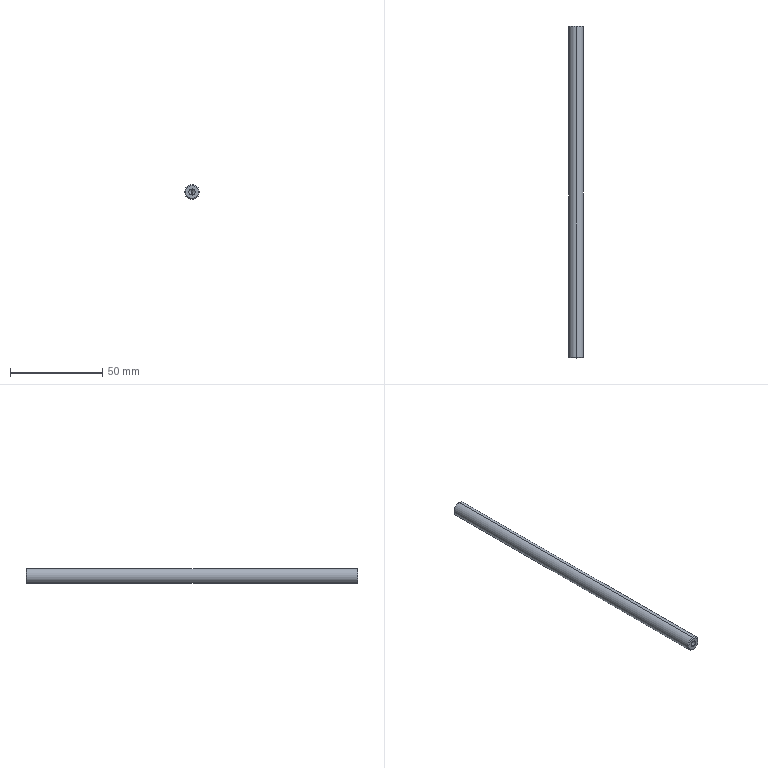Part | STEP file | 04-22 guide post | 1 solid | 12 faces | box 8 x 180 x 8 mm | volume 8953 mm3 | cone 6 | cylinder 4 | plane 2 | commonest cylinder face diameters 3.3 x2 8 x2
STEP:
#1=CARTESIAN_POINT('',(0.,180.,3.5));
#2=VERTEX_POINT('',#1);
#3=CARTESIAN_POINT('',(0.,180.,-3.5));
#4=VERTEX_POINT('',#3);
#5=CARTESIAN_POINT('',(0.,180.,0.));
#6=DIRECTION('',(0.,1.,0.));
#7=DIRECTION('',(0.,0.,1.));
#8=AXIS2_PLACEMENT_3D('',#5,#6,#7);
#9=CIRCLE('',#8,3.5);
#10=EDGE_CURVE('',#2,#4,#9,.T.);
#11=ORIENTED_EDGE('',*,*,#10,.F.);
#12=CARTESIAN_POINT('',(0.,179.5,4.));
#13=VERTEX_POINT('',#12);
#14=CARTESIAN_POINT('',(0.,180.,3.5));
#15=DIRECTION('',(0.,-0.7071,0.7071));
#16=VECTOR('',#15,1000.);
#17=LINE('',#14,#16);
#18=EDGE_CURVE('',#2,#13,#17,.T.);
#19=ORIENTED_EDGE('',*,*,#18,.T.);
#20=CARTESIAN_POINT('',(0.,179.5,-4.));
#21=VERTEX_POINT('',#20);
#22=CARTESIAN_POINT('',(0.,179.5,0.));
#23=DIRECTION('',(0.,-1.,0.));
#24=DIRECTION('',(0.,0.,1.));
#25=AXIS2_PLACEMENT_3D('',#22,#23,#24);
#26=CIRCLE('',#25,4.);
#27=EDGE_CURVE('',#21,#13,#26,.T.);
#28=ORIENTED_EDGE('',*,*,#27,.F.);
#29=CARTESIAN_POINT('',(0.,180.,-3.5));
#30=DIRECTION('',(0.,-0.7071,-0.7071));
#31=VECTOR('',#30,1000.);
#32=LINE('',#29,#31);
#33=EDGE_CURVE('',#4,#21,#32,.T.);
#34=ORIENTED_EDGE('',*,*,#33,.F.);
#35=EDGE_LOOP('',(#11,#19,#28,#34));
#36=FACE_OUTER_BOUND('',#35,.T.);
#37=CARTESIAN_POINT('',(0.,180.,0.));
#38=DIRECTION('',(0.,-1.,0.));
#39=DIRECTION('',(0.,0.,-1.));
#40=AXIS2_PLACEMENT_3D('',#37,#38,#39);
#41=CONICAL_SURFACE('',#40,3.5,0.7854);
#42=ADVANCED_FACE('',(#36),#41,.T.);
#43=CARTESIAN_POINT('',(0.,0.,-3.5));
#44=VERTEX_POINT('',#43);
#45=CARTESIAN_POINT('',(0.,0.,3.5));
#46=VERTEX_POINT('',#45);
#47=CARTESIAN_POINT('',(0.,0.,0.));
#48=DIRECTION('',(0.,-1.,0.));
#49=DIRECTION('',(0.,0.,1.));
#50=AXIS2_PLACEMENT_3D('',#47,#48,#49);
#51=CIRCLE('',#50,3.5);
#52=EDGE_CURVE('',#44,#46,#51,.T.);
#53=ORIENTED_EDGE('',*,*,#52,.F.);
#54=CARTESIAN_POINT('',(0.,0.5,-4.));
#55=VERTEX_POINT('',#54);
#56=CARTESIAN_POINT('',(0.,0.5,-4.));
#57=DIRECTION('',(0.,0.7071,-0.7071));
#58=VECTOR('',#57,1000.);
#59=LINE('',#56,#58);
#60=EDGE_CURVE('',#44,#55,#59,.T.);
#61=ORIENTED_EDGE('',*,*,#60,.T.);
#62=CARTESIAN_POINT('',(0.,0.5,4.));
#63=VERTEX_POINT('',#62);
#64=CARTESIAN_POINT('',(0.,0.5,0.));
#65=DIRECTION('',(0.,1.,0.));
#66=DIRECTION('',(0.,0.,1.));
#67=AXIS2_PLACEMENT_3D('',#64,#65,#66);
#68=CIRCLE('',#67,4.);
#69=EDGE_CURVE('',#63,#55,#68,.T.);
#70=ORIENTED_EDGE('',*,*,#69,.F.);
#71=CARTESIAN_POINT('',(0.,0.5,4.));
#72=DIRECTION('',(0.,0.7071,0.7071));
#73=VECTOR('',#72,1000.);
#74=LINE('',#71,#73);
#75=EDGE_CURVE('',#46,#63,#74,.T.);
#76=ORIENTED_EDGE('',*,*,#75,.F.);
#77=EDGE_LOOP('',(#53,#61,#70,#76));
#78=FACE_OUTER_BOUND('',#77,.T.);
#79=CARTESIAN_POINT('',(0.,0.5,0.));
#80=DIRECTION('',(0.,1.,0.));
#81=DIRECTION('',(0.,0.,1.));
#82=AXIS2_PLACEMENT_3D('',#79,#80,#81);
#83=CONICAL_SURFACE('',#82,4.,0.7854);
#84=ADVANCED_FACE('',(#78),#83,.T.);
#85=CARTESIAN_POINT('',(0.,10.1,1.65));
#86=VERTEX_POINT('',#85);
#87=CARTESIAN_POINT('',(0.,10.1,-1.65));
#88=VERTEX_POINT('',#87);
#89=CARTESIAN_POINT('',(0.,10.1,0.));
#90=DIRECTION('',(0.,-1.,0.));
#91=DIRECTION('',(0.,0.,-1.));
#92=AXIS2_PLACEMENT_3D('',#89,#90,#91);
#93=CIRCLE('',#92,1.65);
#94=EDGE_CURVE('',#86,#88,#93,.T.);
#95=ORIENTED_EDGE('',*,*,#94,.F.);
#96=CARTESIAN_POINT('',(0.,0.,1.65));
#97=VERTEX_POINT('',#96);
#98=CARTESIAN_POINT('',(0.,0.,1.65));
#99=DIRECTION('',(0.,-1.,0.));
#100=VECTOR('',#99,1000.);
#101=LINE('',#98,#100);
#102=EDGE_CURVE('',#86,#97,#101,.T.);
#103=ORIENTED_EDGE('',*,*,#102,.T.);
#104=CARTESIAN_POINT('',(0.,0.,-1.65));
#105=VERTEX_POINT('',#104);
#106=CARTESIAN_POINT('',(0.,0.,0.));
#107=DIRECTION('',(0.,-1.,0.));
#108=DIRECTION('',(0.,0.,-1.));
#109=AXIS2_PLACEMENT_3D('',#106,#107,#108);
#110=CIRCLE('',#109,1.65);
#111=EDGE_CURVE('',#97,#105,#110,.T.);
#112=ORIENTED_EDGE('',*,*,#111,.T.);
#113=CARTESIAN_POINT('',(0.,0.,-1.65));
#114=DIRECTION('',(0.,-1.,0.));
#115=VECTOR('',#114,1000.);
#116=LINE('',#113,#115);
#117=EDGE_CURVE('',#88,#105,#116,.T.);
#118=ORIENTED_EDGE('',*,*,#117,.F.);
#119=EDGE_LOOP('',(#95,#103,#112,#118));
#120=FACE_OUTER_BOUND('',#119,.T.);
#121=CARTESIAN_POINT('',(0.,0.,0.));
#122=DIRECTION('',(0.,-1.,0.));
#123=DIRECTION('',(0.,0.,-1.));
#124=AXIS2_PLACEMENT_3D('',#121,#122,#123);
#125=CYLINDRICAL_SURFACE('',#124,1.65);
#126=ADVANCED_FACE('',(#120),#125,.F.);
#127=CARTESIAN_POINT('',(0.,11.091,0.));
#128=VERTEX_POINT('',#127);
#129=CARTESIAN_POINT('',(0.,10.1,-1.65));
#130=DIRECTION('',(0.,-0.515,-0.8572));
#131=VECTOR('',#130,1000.);
#132=LINE('',#129,#131);
#133=EDGE_CURVE('',#128,#88,#132,.T.);
#134=ORIENTED_EDGE('',*,*,#133,.F.);
#135=CARTESIAN_POINT('',(0.,10.1,1.65));
#136=DIRECTION('',(0.,-0.515,0.8572));
#137=VECTOR('',#136,1000.);
#138=LINE('',#135,#137);
#139=EDGE_CURVE('',#128,#86,#138,.T.);
#140=ORIENTED_EDGE('',*,*,#139,.T.);
#141=ORIENTED_EDGE('',*,*,#94,.T.);
#142=EDGE_LOOP('',(#134,#140,#141));
#143=FACE_OUTER_BOUND('',#142,.T.);
#144=CARTESIAN_POINT('',(0.,10.1,0.));
#145=DIRECTION('',(0.,-1.,0.));
#146=DIRECTION('',(0.,0.,-1.));
#147=AXIS2_PLACEMENT_3D('',#144,#145,#146);
#148=CONICAL_SURFACE('',#147,1.65,1.03);
#149=ADVANCED_FACE('',(#143),#148,.F.);
#150=ORIENTED_EDGE('',*,*,#27,.T.);
#151=CARTESIAN_POINT('',(0.,180.,4.));
#152=DIRECTION('',(0.,-1.,0.));
#153=VECTOR('',#152,1000.);
#154=LINE('',#151,#153);
#155=EDGE_CURVE('',#13,#63,#154,.T.);
#156=ORIENTED_EDGE('',*,*,#155,.T.);
#157=ORIENTED_EDGE('',*,*,#69,.T.);
#158=CARTESIAN_POINT('',(0.,180.,-4.));
#159=DIRECTION('',(0.,-1.,0.));
#160=VECTOR('',#159,1000.);
#161=LINE('',#158,#160);
#162=EDGE_CURVE('',#21,#55,#161,.T.);
#163=ORIENTED_EDGE('',*,*,#162,.F.);
#164=EDGE_LOOP('',(#150,#156,#157,#163));
#165=FACE_OUTER_BOUND('',#164,.T.);
#166=CARTESIAN_POINT('',(0.,180.,0.));
#167=DIRECTION('',(0.,-1.,0.));
#168=DIRECTION('',(0.,0.,-1.));
#169=AXIS2_PLACEMENT_3D('',#166,#167,#168);
#170=CYLINDRICAL_SURFACE('',#169,4.);
#171=ADVANCED_FACE('',(#165),#170,.T.);
#172=ORIENTED_EDGE('',*,*,#155,.F.);
#173=CARTESIAN_POINT('',(0.,179.5,0.));
#174=DIRECTION('',(0.,-1.,0.));
#175=DIRECTION('',(0.,0.,1.));
#176=AXIS2_PLACEMENT_3D('',#173,#174,#175);
#177=CIRCLE('',#176,4.);
#178=EDGE_CURVE('',#13,#21,#177,.T.);
#179=ORIENTED_EDGE('',*,*,#178,.T.);
#180=ORIENTED_EDGE('',*,*,#162,.T.);
#181=CARTESIAN_POINT('',(0.,0.5,0.));
#182=DIRECTION('',(0.,1.,0.));
#183=DIRECTION('',(0.,0.,1.));
#184=AXIS2_PLACEMENT_3D('',#181,#182,#183);
#185=CIRCLE('',#184,4.);
#186=EDGE_CURVE('',#55,#63,#185,.T.);
#187=ORIENTED_EDGE('',*,*,#186,.T.);
#188=EDGE_LOOP('',(#172,#179,#180,#187));
#189=FACE_OUTER_BOUND('',#188,.T.);
#190=CARTESIAN_POINT('',(0.,180.,0.));
#191=DIRECTION('',(0.,-1.,0.));
#192=DIRECTION('',(0.,0.,-1.));
#193=AXIS2_PLACEMENT_3D('',#190,#191,#192);
#194=CYLINDRICAL_SURFACE('',#193,4.);
#195=ADVANCED_FACE('',(#189),#194,.T.);
#196=CARTESIAN_POINT('',(0.,180.,0.));
#197=DIRECTION('',(0.,1.,0.));
#198=DIRECTION('',(0.,0.,1.));
#199=AXIS2_PLACEMENT_3D('',#196,#197,#198);
#200=CIRCLE('',#199,3.5);
#201=EDGE_CURVE('',#4,#2,#200,.T.);
#202=ORIENTED_EDGE('',*,*,#201,.T.);
#203=ORIENTED_EDGE('',*,*,#10,.T.);
#204=EDGE_LOOP('',(#202,#203));
#205=FACE_OUTER_BOUND('',#204,.T.);
#206=CARTESIAN_POINT('',(0.,180.,0.));
#207=DIRECTION('',(0.,1.,0.));
#208=DIRECTION('',(0.,0.,1.));
#209=AXIS2_PLACEMENT_3D('',#206,#207,#208);
#210=PLANE('',#209);
#211=ADVANCED_FACE('',(#205),#210,.T.);
#212=CARTESIAN_POINT('',(0.,0.,0.));
#213=DIRECTION('',(0.,-1.,0.));
#214=DIRECTION('',(0.,0.,1.));
#215=AXIS2_PLACEMENT_3D('',#212,#213,#214);
#216=CIRCLE('',#215,3.5);
#217=EDGE_CURVE('',#46,#44,#216,.T.);
#218=ORIENTED_EDGE('',*,*,#217,.T.);
#219=ORIENTED_EDGE('',*,*,#52,.T.);
#220=EDGE_LOOP('',(#218,#219));
#221=FACE_OUTER_BOUND('',#220,.T.);
#222=CARTESIAN_POINT('',(0.,0.,0.));
#223=DIRECTION('',(0.,-1.,0.));
#224=DIRECTION('',(0.,0.,-1.));
#225=AXIS2_PLACEMENT_3D('',#222,#223,#224);
#226=CIRCLE('',#225,1.65);
#227=EDGE_CURVE('',#105,#97,#226,.T.);
#228=ORIENTED_EDGE('',*,*,#227,.F.);
#229=ORIENTED_EDGE('',*,*,#111,.F.);
#230=EDGE_LOOP('',(#228,#229));
#231=FACE_BOUND('',#230,.T.);
#232=CARTESIAN_POINT('',(0.,0.,0.));
#233=DIRECTION('',(0.,1.,0.));
#234=DIRECTION('',(0.,0.,1.));
#235=AXIS2_PLACEMENT_3D('',#232,#233,#234);
#236=PLANE('',#235);
#237=ADVANCED_FACE('',(#221,#231),#236,.F.);
#238=ORIENTED_EDGE('',*,*,#139,.F.);
#239=ORIENTED_EDGE('',*,*,#133,.T.);
#240=CARTESIAN_POINT('',(0.,10.1,0.));
#241=DIRECTION('',(0.,-1.,0.));
#242=DIRECTION('',(0.,0.,-1.));
#243=AXIS2_PLACEMENT_3D('',#240,#241,#242);
#244=CIRCLE('',#243,1.65);
#245=EDGE_CURVE('',#88,#86,#244,.T.);
#246=ORIENTED_EDGE('',*,*,#245,.T.);
#247=EDGE_LOOP('',(#238,#239,#246));
#248=FACE_OUTER_BOUND('',#247,.T.);
#249=CARTESIAN_POINT('',(0.,10.1,0.));
#250=DIRECTION('',(0.,-1.,0.));
#251=DIRECTION('',(0.,0.,-1.));
#252=AXIS2_PLACEMENT_3D('',#249,#250,#251);
#253=CONICAL_SURFACE('',#252,1.65,1.03);
#254=ADVANCED_FACE('',(#248),#253,.F.);
#255=ORIENTED_EDGE('',*,*,#102,.F.);
#256=ORIENTED_EDGE('',*,*,#245,.F.);
#257=ORIENTED_EDGE('',*,*,#117,.T.);
#258=ORIENTED_EDGE('',*,*,#227,.T.);
#259=EDGE_LOOP('',(#255,#256,#257,#258));
#260=FACE_OUTER_BOUND('',#259,.T.);
#261=CARTESIAN_POINT('',(0.,0.,0.));
#262=DIRECTION('',(0.,-1.,0.));
#263=DIRECTION('',(0.,0.,-1.));
#264=AXIS2_PLACEMENT_3D('',#261,#262,#263);
#265=CYLINDRICAL_SURFACE('',#264,1.65);
#266=ADVANCED_FACE('',(#260),#265,.F.);
#267=ORIENTED_EDGE('',*,*,#60,.F.);
#268=ORIENTED_EDGE('',*,*,#217,.F.);
#269=ORIENTED_EDGE('',*,*,#75,.T.);
#270=ORIENTED_EDGE('',*,*,#186,.F.);
#271=EDGE_LOOP('',(#267,#268,#269,#270));
#272=FACE_OUTER_BOUND('',#271,.T.);
#273=CARTESIAN_POINT('',(0.,0.5,0.));
#274=DIRECTION('',(0.,1.,0.));
#275=DIRECTION('',(0.,0.,1.));
#276=AXIS2_PLACEMENT_3D('',#273,#274,#275);
#277=CONICAL_SURFACE('',#276,4.,0.7854);
#278=ADVANCED_FACE('',(#272),#277,.T.);
#279=ORIENTED_EDGE('',*,*,#18,.F.);
#280=ORIENTED_EDGE('',*,*,#201,.F.);
#281=ORIENTED_EDGE('',*,*,#33,.T.);
#282=ORIENTED_EDGE('',*,*,#178,.F.);
#283=EDGE_LOOP('',(#279,#280,#281,#282));
#284=FACE_OUTER_BOUND('',#283,.T.);
#285=CARTESIAN_POINT('',(0.,180.,0.));
#286=DIRECTION('',(0.,-1.,0.));
#287=DIRECTION('',(0.,0.,-1.));
#288=AXIS2_PLACEMENT_3D('',#285,#286,#287);
#289=CONICAL_SURFACE('',#288,3.5,0.7854);
#290=ADVANCED_FACE('',(#284),#289,.T.);
#291=CLOSED_SHELL('',(#42,#84,#126,#149,#171,#195,#211,#237,#254,#266,#278,#290));
#292=MANIFOLD_SOLID_BREP('',#291);
#293=CARTESIAN_POINT('',(0.,0.,0.));
#294=DIRECTION('',(0.,0.,1.));
#295=DIRECTION('',(1.,0.,0.));
#296=AXIS2_PLACEMENT_3D('',#293,#294,#295);
#297=(LENGTH_UNIT()NAMED_UNIT(*)SI_UNIT(.MILLI.,.METRE.));
#298=UNCERTAINTY_MEASURE_WITH_UNIT(LENGTH_MEASURE(0.00001),#297,'','');
#299=(NAMED_UNIT(*)PLANE_ANGLE_UNIT()SI_UNIT($,.RADIAN.));
#300=(NAMED_UNIT(*)SI_UNIT($,.STERADIAN.)SOLID_ANGLE_UNIT());
#301=(GEOMETRIC_REPRESENTATION_CONTEXT(3)GLOBAL_UNCERTAINTY_ASSIGNED_CONTEXT((#298))GLOBAL_UNIT_ASSIGNED_CONTEXT((#297,#299,#300))REPRESENTATION_CONTEXT('',''));
#302=ADVANCED_BREP_SHAPE_REPRESENTATION('',(#292,#296),#301);